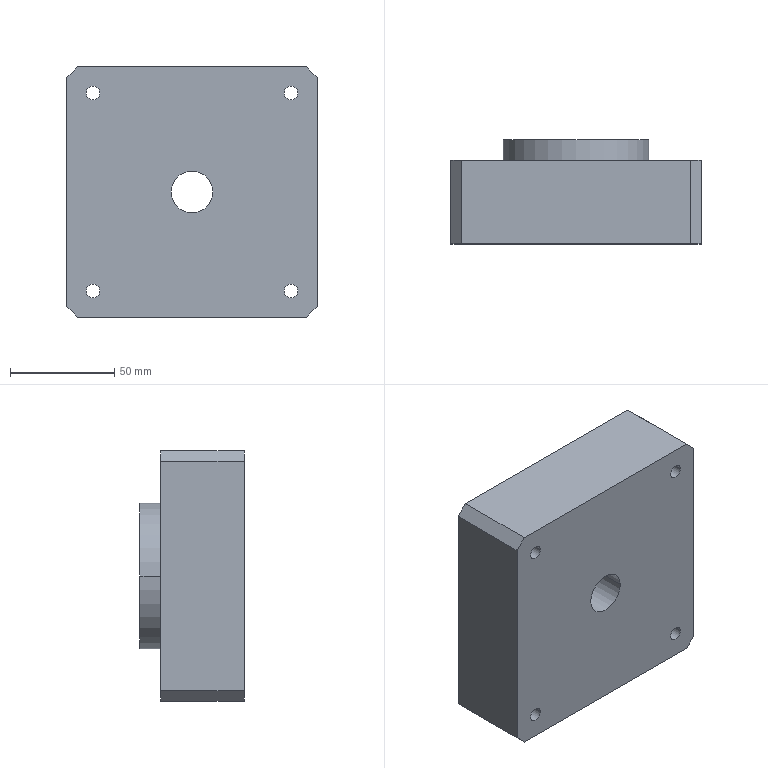Part | STEP file | M6 六角头Screw的柱形沉头Hole 1 | 1 solid | 50 faces | box 120 x 50 x 120 mm | volume 583267 mm3 | cylinder 30 | plane 20 | commonest cylinder face diameters 6 x8 6.6 x8 14.55 x8 20 x2 40 x2 70 x2
STEP:
#1=CARTESIAN_POINT('',(-1528.963,1730.114,2864.251));
#2=VERTEX_POINT('',#1);
#3=CARTESIAN_POINT('',(-1543.513,1730.114,2864.251));
#4=VERTEX_POINT('',#3);
#5=CARTESIAN_POINT('',(-1536.238,1730.114,2864.251));
#6=DIRECTION('',(0.,1.,0.));
#7=DIRECTION('',(-1.,0.,0.));
#8=AXIS2_PLACEMENT_3D('',#5,#6,#7);
#9=CIRCLE('',#8,7.275);
#10=EDGE_CURVE('',#2,#4,#9,.T.);
#11=ORIENTED_EDGE('',*,*,#10,.F.);
#12=CARTESIAN_POINT('',(-1528.963,1734.264,2864.251));
#13=VERTEX_POINT('',#12);
#14=CARTESIAN_POINT('',(-1528.963,1734.264,2864.251));
#15=DIRECTION('',(0.,1.,0.));
#16=VECTOR('',#15,1000.);
#17=LINE('',#14,#16);
#18=EDGE_CURVE('',#2,#13,#17,.T.);
#19=ORIENTED_EDGE('',*,*,#18,.T.);
#20=CARTESIAN_POINT('',(-1543.513,1734.264,2864.251));
#21=VERTEX_POINT('',#20);
#22=CARTESIAN_POINT('',(-1536.238,1734.264,2864.251));
#23=DIRECTION('',(0.,1.,0.));
#24=DIRECTION('',(-1.,0.,0.));
#25=AXIS2_PLACEMENT_3D('',#22,#23,#24);
#26=CIRCLE('',#25,7.275);
#27=EDGE_CURVE('',#13,#21,#26,.T.);
#28=ORIENTED_EDGE('',*,*,#27,.T.);
#29=CARTESIAN_POINT('',(-1543.513,1734.264,2864.251));
#30=DIRECTION('',(0.,1.,0.));
#31=VECTOR('',#30,1000.);
#32=LINE('',#29,#31);
#33=EDGE_CURVE('',#4,#21,#32,.T.);
#34=ORIENTED_EDGE('',*,*,#33,.F.);
#35=EDGE_LOOP('',(#11,#19,#28,#34));
#36=FACE_OUTER_BOUND('',#35,.T.);
#37=CARTESIAN_POINT('',(-1536.238,1734.264,2864.251));
#38=DIRECTION('',(0.,1.,0.));
#39=DIRECTION('',(1.,0.,0.));
#40=AXIS2_PLACEMENT_3D('',#37,#38,#39);
#41=CYLINDRICAL_SURFACE('',#40,7.275);
#42=ADVANCED_FACE('',(#36),#41,.F.);
#43=CARTESIAN_POINT('',(-1532.938,1694.264,2864.251));
#44=VERTEX_POINT('',#43);
#45=CARTESIAN_POINT('',(-1539.538,1694.264,2864.251));
#46=VERTEX_POINT('',#45);
#47=CARTESIAN_POINT('',(-1536.238,1694.264,2864.251));
#48=DIRECTION('',(0.,1.,0.));
#49=DIRECTION('',(-1.,0.,0.));
#50=AXIS2_PLACEMENT_3D('',#47,#48,#49);
#51=CIRCLE('',#50,3.3);
#52=EDGE_CURVE('',#44,#46,#51,.T.);
#53=ORIENTED_EDGE('',*,*,#52,.F.);
#54=CARTESIAN_POINT('',(-1532.938,1730.114,2864.251));
#55=VERTEX_POINT('',#54);
#56=CARTESIAN_POINT('',(-1532.938,1734.264,2864.251));
#57=DIRECTION('',(0.,1.,0.));
#58=VECTOR('',#57,1000.);
#59=LINE('',#56,#58);
#60=EDGE_CURVE('',#44,#55,#59,.T.);
#61=ORIENTED_EDGE('',*,*,#60,.T.);
#62=CARTESIAN_POINT('',(-1539.538,1730.114,2864.251));
#63=VERTEX_POINT('',#62);
#64=CARTESIAN_POINT('',(-1536.238,1730.114,2864.251));
#65=DIRECTION('',(0.,1.,0.));
#66=DIRECTION('',(-1.,0.,0.));
#67=AXIS2_PLACEMENT_3D('',#64,#65,#66);
#68=CIRCLE('',#67,3.3);
#69=EDGE_CURVE('',#55,#63,#68,.T.);
#70=ORIENTED_EDGE('',*,*,#69,.T.);
#71=CARTESIAN_POINT('',(-1539.538,1734.264,2864.251));
#72=DIRECTION('',(0.,1.,0.));
#73=VECTOR('',#72,1000.);
#74=LINE('',#71,#73);
#75=EDGE_CURVE('',#46,#63,#74,.T.);
#76=ORIENTED_EDGE('',*,*,#75,.F.);
#77=EDGE_LOOP('',(#53,#61,#70,#76));
#78=FACE_OUTER_BOUND('',#77,.T.);
#79=CARTESIAN_POINT('',(-1536.238,1734.264,2864.251));
#80=DIRECTION('',(0.,1.,0.));
#81=DIRECTION('',(1.,0.,0.));
#82=AXIS2_PLACEMENT_3D('',#79,#80,#81);
#83=CYLINDRICAL_SURFACE('',#82,3.3);
#84=ADVANCED_FACE('',(#78),#83,.F.);
#85=CARTESIAN_POINT('',(-1433.963,1730.114,2769.251));
#86=VERTEX_POINT('',#85);
#87=CARTESIAN_POINT('',(-1448.513,1730.114,2769.251));
#88=VERTEX_POINT('',#87);
#89=CARTESIAN_POINT('',(-1441.238,1730.114,2769.251));
#90=DIRECTION('',(0.,1.,0.));
#91=DIRECTION('',(-1.,0.,0.));
#92=AXIS2_PLACEMENT_3D('',#89,#90,#91);
#93=CIRCLE('',#92,7.275);
#94=EDGE_CURVE('',#86,#88,#93,.T.);
#95=ORIENTED_EDGE('',*,*,#94,.F.);
#96=CARTESIAN_POINT('',(-1433.963,1734.264,2769.251));
#97=VERTEX_POINT('',#96);
#98=CARTESIAN_POINT('',(-1433.963,1734.264,2769.251));
#99=DIRECTION('',(0.,1.,0.));
#100=VECTOR('',#99,1000.);
#101=LINE('',#98,#100);
#102=EDGE_CURVE('',#86,#97,#101,.T.);
#103=ORIENTED_EDGE('',*,*,#102,.T.);
#104=CARTESIAN_POINT('',(-1448.513,1734.264,2769.251));
#105=VERTEX_POINT('',#104);
#106=CARTESIAN_POINT('',(-1441.238,1734.264,2769.251));
#107=DIRECTION('',(0.,1.,0.));
#108=DIRECTION('',(-1.,0.,0.));
#109=AXIS2_PLACEMENT_3D('',#106,#107,#108);
#110=CIRCLE('',#109,7.275);
#111=EDGE_CURVE('',#97,#105,#110,.T.);
#112=ORIENTED_EDGE('',*,*,#111,.T.);
#113=CARTESIAN_POINT('',(-1448.513,1734.264,2769.251));
#114=DIRECTION('',(0.,1.,0.));
#115=VECTOR('',#114,1000.);
#116=LINE('',#113,#115);
#117=EDGE_CURVE('',#88,#105,#116,.T.);
#118=ORIENTED_EDGE('',*,*,#117,.F.);
#119=EDGE_LOOP('',(#95,#103,#112,#118));
#120=FACE_OUTER_BOUND('',#119,.T.);
#121=CARTESIAN_POINT('',(-1441.238,1734.264,2769.251));
#122=DIRECTION('',(0.,1.,0.));
#123=DIRECTION('',(1.,0.,0.));
#124=AXIS2_PLACEMENT_3D('',#121,#122,#123);
#125=CYLINDRICAL_SURFACE('',#124,7.275);
#126=ADVANCED_FACE('',(#120),#125,.F.);
#127=CARTESIAN_POINT('',(-1437.938,1694.264,2769.251));
#128=VERTEX_POINT('',#127);
#129=CARTESIAN_POINT('',(-1444.538,1694.264,2769.251));
#130=VERTEX_POINT('',#129);
#131=CARTESIAN_POINT('',(-1441.238,1694.264,2769.251));
#132=DIRECTION('',(0.,1.,0.));
#133=DIRECTION('',(-1.,0.,0.));
#134=AXIS2_PLACEMENT_3D('',#131,#132,#133);
#135=CIRCLE('',#134,3.3);
#136=EDGE_CURVE('',#128,#130,#135,.T.);
#137=ORIENTED_EDGE('',*,*,#136,.F.);
#138=CARTESIAN_POINT('',(-1437.938,1730.114,2769.251));
#139=VERTEX_POINT('',#138);
#140=CARTESIAN_POINT('',(-1437.938,1734.264,2769.251));
#141=DIRECTION('',(0.,1.,0.));
#142=VECTOR('',#141,1000.);
#143=LINE('',#140,#142);
#144=EDGE_CURVE('',#128,#139,#143,.T.);
#145=ORIENTED_EDGE('',*,*,#144,.T.);
#146=CARTESIAN_POINT('',(-1444.538,1730.114,2769.251));
#147=VERTEX_POINT('',#146);
#148=CARTESIAN_POINT('',(-1441.238,1730.114,2769.251));
#149=DIRECTION('',(0.,1.,0.));
#150=DIRECTION('',(-1.,0.,0.));
#151=AXIS2_PLACEMENT_3D('',#148,#149,#150);
#152=CIRCLE('',#151,3.3);
#153=EDGE_CURVE('',#139,#147,#152,.T.);
#154=ORIENTED_EDGE('',*,*,#153,.T.);
#155=CARTESIAN_POINT('',(-1444.538,1734.264,2769.251));
#156=DIRECTION('',(0.,1.,0.));
#157=VECTOR('',#156,1000.);
#158=LINE('',#155,#157);
#159=EDGE_CURVE('',#130,#147,#158,.T.);
#160=ORIENTED_EDGE('',*,*,#159,.F.);
#161=EDGE_LOOP('',(#137,#145,#154,#160));
#162=FACE_OUTER_BOUND('',#161,.T.);
#163=CARTESIAN_POINT('',(-1441.238,1734.264,2769.251));
#164=DIRECTION('',(0.,1.,0.));
#165=DIRECTION('',(1.,0.,0.));
#166=AXIS2_PLACEMENT_3D('',#163,#164,#165);
#167=CYLINDRICAL_SURFACE('',#166,3.3);
#168=ADVANCED_FACE('',(#162),#167,.F.);
#169=CARTESIAN_POINT('',(-1433.963,1730.114,2864.251));
#170=VERTEX_POINT('',#169);
#171=CARTESIAN_POINT('',(-1448.513,1730.114,2864.251));
#172=VERTEX_POINT('',#171);
#173=CARTESIAN_POINT('',(-1441.238,1730.114,2864.251));
#174=DIRECTION('',(0.,1.,0.));
#175=DIRECTION('',(-1.,0.,0.));
#176=AXIS2_PLACEMENT_3D('',#173,#174,#175);
#177=CIRCLE('',#176,7.275);
#178=EDGE_CURVE('',#170,#172,#177,.T.);
#179=ORIENTED_EDGE('',*,*,#178,.F.);
#180=CARTESIAN_POINT('',(-1433.963,1734.264,2864.251));
#181=VERTEX_POINT('',#180);
#182=CARTESIAN_POINT('',(-1433.963,1734.264,2864.251));
#183=DIRECTION('',(0.,1.,0.));
#184=VECTOR('',#183,1000.);
#185=LINE('',#182,#184);
#186=EDGE_CURVE('',#170,#181,#185,.T.);
#187=ORIENTED_EDGE('',*,*,#186,.T.);
#188=CARTESIAN_POINT('',(-1448.513,1734.264,2864.251));
#189=VERTEX_POINT('',#188);
#190=CARTESIAN_POINT('',(-1441.238,1734.264,2864.251));
#191=DIRECTION('',(0.,1.,0.));
#192=DIRECTION('',(-1.,0.,0.));
#193=AXIS2_PLACEMENT_3D('',#190,#191,#192);
#194=CIRCLE('',#193,7.275);
#195=EDGE_CURVE('',#181,#189,#194,.T.);
#196=ORIENTED_EDGE('',*,*,#195,.T.);
#197=CARTESIAN_POINT('',(-1448.513,1734.264,2864.251));
#198=DIRECTION('',(0.,1.,0.));
#199=VECTOR('',#198,1000.);
#200=LINE('',#197,#199);
#201=EDGE_CURVE('',#172,#189,#200,.T.);
#202=ORIENTED_EDGE('',*,*,#201,.F.);
#203=EDGE_LOOP('',(#179,#187,#196,#202));
#204=FACE_OUTER_BOUND('',#203,.T.);
#205=CARTESIAN_POINT('',(-1441.238,1734.264,2864.251));
#206=DIRECTION('',(0.,1.,0.));
#207=DIRECTION('',(1.,0.,0.));
#208=AXIS2_PLACEMENT_3D('',#205,#206,#207);
#209=CYLINDRICAL_SURFACE('',#208,7.275);
#210=ADVANCED_FACE('',(#204),#209,.F.);
#211=CARTESIAN_POINT('',(-1437.938,1694.264,2864.251));
#212=VERTEX_POINT('',#211);
#213=CARTESIAN_POINT('',(-1444.538,1694.264,2864.251));
#214=VERTEX_POINT('',#213);
#215=CARTESIAN_POINT('',(-1441.238,1694.264,2864.251));
#216=DIRECTION('',(0.,1.,0.));
#217=DIRECTION('',(-1.,0.,0.));
#218=AXIS2_PLACEMENT_3D('',#215,#216,#217);
#219=CIRCLE('',#218,3.3);
#220=EDGE_CURVE('',#212,#214,#219,.T.);
#221=ORIENTED_EDGE('',*,*,#220,.F.);
#222=CARTESIAN_POINT('',(-1437.938,1730.114,2864.251));
#223=VERTEX_POINT('',#222);
#224=CARTESIAN_POINT('',(-1437.938,1734.264,2864.251));
#225=DIRECTION('',(0.,1.,0.));
#226=VECTOR('',#225,1000.);
#227=LINE('',#224,#226);
#228=EDGE_CURVE('',#212,#223,#227,.T.);
#229=ORIENTED_EDGE('',*,*,#228,.T.);
#230=CARTESIAN_POINT('',(-1444.538,1730.114,2864.251));
#231=VERTEX_POINT('',#230);
#232=CARTESIAN_POINT('',(-1441.238,1730.114,2864.251));
#233=DIRECTION('',(0.,1.,0.));
#234=DIRECTION('',(-1.,0.,0.));
#235=AXIS2_PLACEMENT_3D('',#232,#233,#234);
#236=CIRCLE('',#235,3.3);
#237=EDGE_CURVE('',#223,#231,#236,.T.);
#238=ORIENTED_EDGE('',*,*,#237,.T.);
#239=CARTESIAN_POINT('',(-1444.538,1734.264,2864.251));
#240=DIRECTION('',(0.,1.,0.));
#241=VECTOR('',#240,1000.);
#242=LINE('',#239,#241);
#243=EDGE_CURVE('',#214,#231,#242,.T.);
#244=ORIENTED_EDGE('',*,*,#243,.F.);
#245=EDGE_LOOP('',(#221,#229,#238,#244));
#246=FACE_OUTER_BOUND('',#245,.T.);
#247=CARTESIAN_POINT('',(-1441.238,1734.264,2864.251));
#248=DIRECTION('',(0.,1.,0.));
#249=DIRECTION('',(1.,0.,0.));
#250=AXIS2_PLACEMENT_3D('',#247,#248,#249);
#251=CYLINDRICAL_SURFACE('',#250,3.3);
#252=ADVANCED_FACE('',(#246),#251,.F.);
#253=CARTESIAN_POINT('',(-1528.963,1730.114,2769.251));
#254=VERTEX_POINT('',#253);
#255=CARTESIAN_POINT('',(-1543.513,1730.114,2769.251));
#256=VERTEX_POINT('',#255);
#257=CARTESIAN_POINT('',(-1536.238,1730.114,2769.251));
#258=DIRECTION('',(0.,1.,0.));
#259=DIRECTION('',(-1.,0.,0.));
#260=AXIS2_PLACEMENT_3D('',#257,#258,#259);
#261=CIRCLE('',#260,7.275);
#262=EDGE_CURVE('',#254,#256,#261,.T.);
#263=ORIENTED_EDGE('',*,*,#262,.F.);
#264=CARTESIAN_POINT('',(-1528.963,1734.264,2769.251));
#265=VERTEX_POINT('',#264);
#266=CARTESIAN_POINT('',(-1528.963,1734.264,2769.251));
#267=DIRECTION('',(0.,1.,0.));
#268=VECTOR('',#267,1000.);
#269=LINE('',#266,#268);
#270=EDGE_CURVE('',#254,#265,#269,.T.);
#271=ORIENTED_EDGE('',*,*,#270,.T.);
#272=CARTESIAN_POINT('',(-1543.513,1734.264,2769.251));
#273=VERTEX_POINT('',#272);
#274=CARTESIAN_POINT('',(-1536.238,1734.264,2769.251));
#275=DIRECTION('',(0.,1.,0.));
#276=DIRECTION('',(-1.,0.,0.));
#277=AXIS2_PLACEMENT_3D('',#274,#275,#276);
#278=CIRCLE('',#277,7.275);
#279=EDGE_CURVE('',#265,#273,#278,.T.);
#280=ORIENTED_EDGE('',*,*,#279,.T.);
#281=CARTESIAN_POINT('',(-1543.513,1734.264,2769.251));
#282=DIRECTION('',(0.,1.,0.));
#283=VECTOR('',#282,1000.);
#284=LINE('',#281,#283);
#285=EDGE_CURVE('',#256,#273,#284,.T.);
#286=ORIENTED_EDGE('',*,*,#285,.F.);
#287=EDGE_LOOP('',(#263,#271,#280,#286));
#288=FACE_OUTER_BOUND('',#287,.T.);
#289=CARTESIAN_POINT('',(-1536.238,1734.264,2769.251));
#290=DIRECTION('',(0.,1.,0.));
#291=DIRECTION('',(1.,0.,0.));
#292=AXIS2_PLACEMENT_3D('',#289,#290,#291);
#293=CYLINDRICAL_SURFACE('',#292,7.275);
#294=ADVANCED_FACE('',(#288),#293,.F.);
#295=CARTESIAN_POINT('',(-1532.938,1694.264,2769.251));
#296=VERTEX_POINT('',#295);
#297=CARTESIAN_POINT('',(-1539.538,1694.264,2769.251));
#298=VERTEX_POINT('',#297);
#299=CARTESIAN_POINT('',(-1536.238,1694.264,2769.251));
#300=DIRECTION('',(0.,1.,0.));
#301=DIRECTION('',(-1.,0.,0.));
#302=AXIS2_PLACEMENT_3D('',#299,#300,#301);
#303=CIRCLE('',#302,3.3);
#304=EDGE_CURVE('',#296,#298,#303,.T.);
#305=ORIENTED_EDGE('',*,*,#304,.F.);
#306=CARTESIAN_POINT('',(-1532.938,1730.114,2769.251));
#307=VERTEX_POINT('',#306);
#308=CARTESIAN_POINT('',(-1532.938,1734.264,2769.251));
#309=DIRECTION('',(0.,1.,0.));
#310=VECTOR('',#309,1000.);
#311=LINE('',#308,#310);
#312=EDGE_CURVE('',#296,#307,#311,.T.);
#313=ORIENTED_EDGE('',*,*,#312,.T.);
#314=CARTESIAN_POINT('',(-1539.538,1730.114,2769.251));
#315=VERTEX_POINT('',#314);
#316=CARTESIAN_POINT('',(-1536.238,1730.114,2769.251));
#317=DIRECTION('',(0.,1.,0.));
#318=DIRECTION('',(-1.,0.,0.));
#319=AXIS2_PLACEMENT_3D('',#316,#317,#318);
#320=CIRCLE('',#319,3.3);
#321=EDGE_CURVE('',#307,#315,#320,.T.);
#322=ORIENTED_EDGE('',*,*,#321,.T.);
#323=CARTESIAN_POINT('',(-1539.538,1734.264,2769.251));
#324=DIRECTION('',(0.,1.,0.));
#325=VECTOR('',#324,1000.);
#326=LINE('',#323,#325);
#327=EDGE_CURVE('',#298,#315,#326,.T.);
#328=ORIENTED_EDGE('',*,*,#327,.F.);
#329=EDGE_LOOP('',(#305,#313,#322,#328));
#330=FACE_OUTER_BOUND('',#329,.T.);
#331=CARTESIAN_POINT('',(-1536.238,1734.264,2769.251));
#332=DIRECTION('',(0.,1.,0.));
#333=DIRECTION('',(1.,0.,0.));
#334=AXIS2_PLACEMENT_3D('',#331,#332,#333);
#335=CYLINDRICAL_SURFACE('',#334,3.3);
#336=ADVANCED_FACE('',(#330),#335,.F.);
#337=CARTESIAN_POINT('',(-1515.738,1724.264,2786.751));
#338=VERTEX_POINT('',#337);
#339=CARTESIAN_POINT('',(-1521.738,1724.264,2786.751));
#340=VERTEX_POINT('',#339);
#341=CARTESIAN_POINT('',(-1518.738,1724.264,2786.751));
#342=DIRECTION('',(0.,1.,0.));
#343=DIRECTION('',(-1.,0.,0.));
#344=AXIS2_PLACEMENT_3D('',#341,#342,#343);
#345=CIRCLE('',#344,3.);
#346=EDGE_CURVE('',#338,#340,#345,.T.);
#347=ORIENTED_EDGE('',*,*,#346,.F.);
#348=CARTESIAN_POINT('',(-1515.738,1734.264,2786.751));
#349=VERTEX_POINT('',#348);
#350=CARTESIAN_POINT('',(-1515.738,1724.264,2786.751));
#351=DIRECTION('',(0.,1.,0.));
#352=VECTOR('',#351,1000.);
#353=LINE('',#350,#352);
#354=EDGE_CURVE('',#338,#349,#353,.T.);
#355=ORIENTED_EDGE('',*,*,#354,.T.);
#356=CARTESIAN_POINT('',(-1521.738,1734.264,2786.751));
#357=VERTEX_POINT('',#356);
#358=CARTESIAN_POINT('',(-1518.738,1734.264,2786.751));
#359=DIRECTION('',(0.,1.,0.));
#360=DIRECTION('',(-1.,0.,0.));
#361=AXIS2_PLACEMENT_3D('',#358,#359,#360);
#362=CIRCLE('',#361,3.);
#363=EDGE_CURVE('',#349,#357,#362,.T.);
#364=ORIENTED_EDGE('',*,*,#363,.T.);
#365=CARTESIAN_POINT('',(-1521.738,1724.264,2786.751));
#366=DIRECTION('',(0.,1.,0.));
#367=VECTOR('',#366,1000.);
#368=LINE('',#365,#367);
#369=EDGE_CURVE('',#340,#357,#368,.T.);
#370=ORIENTED_EDGE('',*,*,#369,.F.);
#371=EDGE_LOOP('',(#347,#355,#364,#370));
#372=FACE_OUTER_BOUND('',#371,.T.);
#373=CARTESIAN_POINT('',(-1518.738,1724.264,2786.751));
#374=DIRECTION('',(0.,1.,0.));
#375=DIRECTION('',(1.,0.,0.));
#376=AXIS2_PLACEMENT_3D('',#373,#374,#375);
#377=CYLINDRICAL_SURFACE('',#376,3.);
#378=ADVANCED_FACE('',(#372),#377,.F.);
#379=CARTESIAN_POINT('',(-1515.738,1724.264,2846.751));
#380=VERTEX_POINT('',#379);
#381=CARTESIAN_POINT('',(-1521.738,1724.264,2846.751));
#382=VERTEX_POINT('',#381);
#383=CARTESIAN_POINT('',(-1518.738,1724.264,2846.751));
#384=DIRECTION('',(0.,1.,0.));
#385=DIRECTION('',(-1.,0.,0.));
#386=AXIS2_PLACEMENT_3D('',#383,#384,#385);
#387=CIRCLE('',#386,3.);
#388=EDGE_CURVE('',#380,#382,#387,.T.);
#389=ORIENTED_EDGE('',*,*,#388,.F.);
#390=CARTESIAN_POINT('',(-1515.738,1734.264,2846.751));
#391=VERTEX_POINT('',#390);
#392=CARTESIAN_POINT('',(-1515.738,1724.264,2846.751));
#393=DIRECTION('',(0.,1.,0.));
#394=VECTOR('',#393,1000.);
#395=LINE('',#392,#394);
#396=EDGE_CURVE('',#380,#391,#395,.T.);
#397=ORIENTED_EDGE('',*,*,#396,.T.);
#398=CARTESIAN_POINT('',(-1521.738,1734.264,2846.751));
#399=VERTEX_POINT('',#398);
#400=CARTESIAN_POINT('',(-1518.738,1734.264,2846.751));
#401=DIRECTION('',(0.,1.,0.));
#402=DIRECTION('',(-1.,0.,0.));
#403=AXIS2_PLACEMENT_3D('',#400,#401,#402);
#404=CIRCLE('',#403,3.);
#405=EDGE_CURVE('',#391,#399,#404,.T.);
#406=ORIENTED_EDGE('',*,*,#405,.T.);
#407=CARTESIAN_POINT('',(-1521.738,1724.264,2846.751));
#408=DIRECTION('',(0.,1.,0.));
#409=VECTOR('',#408,1000.);
#410=LINE('',#407,#409);
#411=EDGE_CURVE('',#382,#399,#410,.T.);
#412=ORIENTED_EDGE('',*,*,#411,.F.);
#413=EDGE_LOOP('',(#389,#397,#406,#412));
#414=FACE_OUTER_BOUND('',#413,.T.);
#415=CARTESIAN_POINT('',(-1518.738,1724.264,2846.751));
#416=DIRECTION('',(0.,1.,0.));
#417=DIRECTION('',(1.,0.,0.));
#418=AXIS2_PLACEMENT_3D('',#415,#416,#417);
#419=CYLINDRICAL_SURFACE('',#418,3.);
#420=ADVANCED_FACE('',(#414),#419,.F.);
#421=CARTESIAN_POINT('',(-1455.738,1724.264,2786.751));
#422=VERTEX_POINT('',#421);
#423=CARTESIAN_POINT('',(-1461.738,1724.264,2786.751));
#424=VERTEX_POINT('',#423);
#425=CARTESIAN_POINT('',(-1458.738,1724.264,2786.751));
#426=DIRECTION('',(0.,1.,0.));
#427=DIRECTION('',(-1.,0.,0.));
#428=AXIS2_PLACEMENT_3D('',#425,#426,#427);
#429=CIRCLE('',#428,3.);
#430=EDGE_CURVE('',#422,#424,#429,.T.);
#431=ORIENTED_EDGE('',*,*,#430,.F.);
#432=CARTESIAN_POINT('',(-1455.738,1734.264,2786.751));
#433=VERTEX_POINT('',#432);
#434=CARTESIAN_POINT('',(-1455.738,1724.264,2786.751));
#435=DIRECTION('',(0.,1.,0.));
#436=VECTOR('',#435,1000.);
#437=LINE('',#434,#436);
#438=EDGE_CURVE('',#422,#433,#437,.T.);
#439=ORIENTED_EDGE('',*,*,#438,.T.);
#440=CARTESIAN_POINT('',(-1461.738,1734.264,2786.751));
#441=VERTEX_POINT('',#440);
#442=CARTESIAN_POINT('',(-1458.738,1734.264,2786.751));
#443=DIRECTION('',(0.,1.,0.));
#444=DIRECTION('',(-1.,0.,0.));
#445=AXIS2_PLACEMENT_3D('',#442,#443,#444);
#446=CIRCLE('',#445,3.);
#447=EDGE_CURVE('',#433,#441,#446,.T.);
#448=ORIENTED_EDGE('',*,*,#447,.T.);
#449=CARTESIAN_POINT('',(-1461.738,1724.264,2786.751));
#450=DIRECTION('',(0.,1.,0.));
#451=VECTOR('',#450,1000.);
#452=LINE('',#449,#451);
#453=EDGE_CURVE('',#424,#441,#452,.T.);
#454=ORIENTED_EDGE('',*,*,#453,.F.);
#455=EDGE_LOOP('',(#431,#439,#448,#454));
#456=FACE_OUTER_BOUND('',#455,.T.);
#457=CARTESIAN_POINT('',(-1458.738,1724.264,2786.751));
#458=DIRECTION('',(0.,1.,0.));
#459=DIRECTION('',(1.,0.,0.));
#460=AXIS2_PLACEMENT_3D('',#457,#458,#459);
#461=CYLINDRICAL_SURFACE('',#460,3.);
#462=ADVANCED_FACE('',(#456),#461,.F.);
#463=CARTESIAN_POINT('',(-1455.738,1724.264,2846.751));
#464=VERTEX_POINT('',#463);
#465=CARTESIAN_POINT('',(-1461.738,1724.264,2846.751));
#466=VERTEX_POINT('',#465);
#467=CARTESIAN_POINT('',(-1458.738,1724.264,2846.751));
#468=DIRECTION('',(0.,1.,0.));
#469=DIRECTION('',(-1.,0.,0.));
#470=AXIS2_PLACEMENT_3D('',#467,#468,#469);
#471=CIRCLE('',#470,3.);
#472=EDGE_CURVE('',#464,#466,#471,.T.);
#473=ORIENTED_EDGE('',*,*,#472,.F.);
#474=CARTESIAN_POINT('',(-1455.738,1734.264,2846.751));
#475=VERTEX_POINT('',#474);
#476=CARTESIAN_POINT('',(-1455.738,1724.264,2846.751));
#477=DIRECTION('',(0.,1.,0.));
#478=VECTOR('',#477,1000.);
#479=LINE('',#476,#478);
#480=EDGE_CURVE('',#464,#475,#479,.T.);
#481=ORIENTED_EDGE('',*,*,#480,.T.);
#482=CARTESIAN_POINT('',(-1461.738,1734.264,2846.751));
#483=VERTEX_POINT('',#482);
#484=CARTESIAN_POINT('',(-1458.738,1734.264,2846.751));
#485=DIRECTION('',(0.,1.,0.));
#486=DIRECTION('',(-1.,0.,0.));
#487=AXIS2_PLACEMENT_3D('',#484,#485,#486);
#488=CIRCLE('',#487,3.);
#489=EDGE_CURVE('',#475,#483,#488,.T.);
#490=ORIENTED_EDGE('',*,*,#489,.T.);
#491=CARTESIAN_POINT('',(-1461.738,1724.264,2846.751));
#492=DIRECTION('',(0.,1.,0.));
#493=VECTOR('',#492,1000.);
#494=LINE('',#491,#493);
#495=EDGE_CURVE('',#466,#483,#494,.T.);
#496=ORIENTED_EDGE('',*,*,#495,.F.);
#497=EDGE_LOOP('',(#473,#481,#490,#496));
#498=FACE_OUTER_BOUND('',#497,.T.);
#499=CARTESIAN_POINT('',(-1458.738,1724.264,2846.751));
#500=DIRECTION('',(0.,1.,0.));
#501=DIRECTION('',(1.,0.,0.));
#502=AXIS2_PLACEMENT_3D('',#499,#500,#501);
#503=CYLINDRICAL_SURFACE('',#502,3.);
#504=ADVANCED_FACE('',(#498),#503,.F.);
#505=CARTESIAN_POINT('',(-1498.738,1694.264,2816.751));
#506=VERTEX_POINT('',#505);
#507=CARTESIAN_POINT('',(-1478.738,1694.264,2816.751));
#508=VERTEX_POINT('',#507);
#509=CARTESIAN_POINT('',(-1488.738,1694.264,2816.751));
#510=DIRECTION('',(0.,-1.,0.));
#511=DIRECTION('',(1.,0.,0.));
#512=AXIS2_PLACEMENT_3D('',#509,#510,#511);
#513=CIRCLE('',#512,10.);
#514=EDGE_CURVE('',#506,#508,#513,.T.);
#515=ORIENTED_EDGE('',*,*,#514,.T.);
#516=CARTESIAN_POINT('',(-1478.738,1739.264,2816.751));
#517=VERTEX_POINT('',#516);
#518=CARTESIAN_POINT('',(-1478.738,1650.264,2816.751));
#519=DIRECTION('',(0.,1.,0.));
#520=VECTOR('',#519,1000.);
#521=LINE('',#518,#520);
#522=EDGE_CURVE('',#508,#517,#521,.T.);
#523=ORIENTED_EDGE('',*,*,#522,.T.);
#524=CARTESIAN_POINT('',(-1498.738,1739.264,2816.751));
#525=VERTEX_POINT('',#524);
#526=CARTESIAN_POINT('',(-1488.738,1739.264,2816.751));
#527=DIRECTION('',(0.,1.,0.));
#528=DIRECTION('',(-1.,0.,0.));
#529=AXIS2_PLACEMENT_3D('',#526,#527,#528);
#530=CIRCLE('',#529,10.);
#531=EDGE_CURVE('',#517,#525,#530,.T.);
#532=ORIENTED_EDGE('',*,*,#531,.T.);
#533=CARTESIAN_POINT('',(-1498.738,1650.264,2816.751));
#534=DIRECTION('',(0.,1.,0.));
#535=VECTOR('',#534,1000.);
#536=LINE('',#533,#535);
#537=EDGE_CURVE('',#506,#525,#536,.T.);
#538=ORIENTED_EDGE('',*,*,#537,.F.);
#539=EDGE_LOOP('',(#515,#523,#532,#538));
#540=FACE_OUTER_BOUND('',#539,.T.);
#541=CARTESIAN_POINT('',(-1488.738,1650.264,2816.751));
#542=DIRECTION('',(0.,1.,0.));
#543=DIRECTION('',(1.,0.,0.));
#544=AXIS2_PLACEMENT_3D('',#541,#542,#543);
#545=CYLINDRICAL_SURFACE('',#544,10.);
#546=ADVANCED_FACE('',(#540),#545,.F.);
#547=CARTESIAN_POINT('',(-1468.738,1739.264,2816.751));
#548=VERTEX_POINT('',#547);
#549=CARTESIAN_POINT('',(-1508.738,1739.264,2816.751));
#550=VERTEX_POINT('',#549);
#551=CARTESIAN_POINT('',(-1488.738,1739.264,2816.751));
#552=DIRECTION('',(0.,1.,0.));
#553=DIRECTION('',(-1.,0.,0.));
#554=AXIS2_PLACEMENT_3D('',#551,#552,#553);
#555=CIRCLE('',#554,20.);
#556=EDGE_CURVE('',#548,#550,#555,.T.);
#557=ORIENTED_EDGE('',*,*,#556,.F.);
#558=CARTESIAN_POINT('',(-1468.738,1744.264,2816.751));
#559=VERTEX_POINT('',#558);
#560=CARTESIAN_POINT('',(-1468.738,1739.264,2816.751));
#561=DIRECTION('',(0.,1.,0.));
#562=VECTOR('',#561,1000.);
#563=LINE('',#560,#562);
#564=EDGE_CURVE('',#548,#559,#563,.T.);
#565=ORIENTED_EDGE('',*,*,#564,.T.);
#566=CARTESIAN_POINT('',(-1508.738,1744.264,2816.751));
#567=VERTEX_POINT('',#566);
#568=CARTESIAN_POINT('',(-1488.738,1744.264,2816.751));
#569=DIRECTION('',(0.,1.,0.));
#570=DIRECTION('',(-1.,0.,0.));
#571=AXIS2_PLACEMENT_3D('',#568,#569,#570);
#572=CIRCLE('',#571,20.);
#573=EDGE_CURVE('',#559,#567,#572,.T.);
#574=ORIENTED_EDGE('',*,*,#573,.T.);
#575=CARTESIAN_POINT('',(-1508.738,1739.264,2816.751));
#576=DIRECTION('',(0.,1.,0.));
#577=VECTOR('',#576,1000.);
#578=LINE('',#575,#577);
#579=EDGE_CURVE('',#550,#567,#578,.T.);
#580=ORIENTED_EDGE('',*,*,#579,.F.);
#581=EDGE_LOOP('',(#557,#565,#574,#580));
#582=FACE_OUTER_BOUND('',#581,.T.);
#583=CARTESIAN_POINT('',(-1488.738,1739.264,2816.751));
#584=DIRECTION('',(0.,1.,0.));
#585=DIRECTION('',(1.,0.,0.));
#586=AXIS2_PLACEMENT_3D('',#583,#584,#585);
#587=CYLINDRICAL_SURFACE('',#586,20.);
#588=ADVANCED_FACE('',(#582),#587,.F.);
#589=CARTESIAN_POINT('',(-1523.738,1744.264,2816.751));
#590=VERTEX_POINT('',#589);
#591=CARTESIAN_POINT('',(-1453.738,1744.264,2816.751));
#592=VERTEX_POINT('',#591);
#593=CARTESIAN_POINT('',(-1488.738,1744.264,2816.751));
#594=DIRECTION('',(0.,1.,0.));
#595=DIRECTION('',(-1.,0.,0.));
#596=AXIS2_PLACEMENT_3D('',#593,#594,#595);
#597=CIRCLE('',#596,35.);
#598=EDGE_CURVE('',#590,#592,#597,.T.);
#599=ORIENTED_EDGE('',*,*,#598,.F.);
#600=CARTESIAN_POINT('',(-1523.738,1734.264,2816.751));
#601=VERTEX_POINT('',#600);
#602=CARTESIAN_POINT('',(-1523.738,1744.264,2816.751));
#603=DIRECTION('',(0.,1.,0.));
#604=VECTOR('',#603,1000.);
#605=LINE('',#602,#604);
#606=EDGE_CURVE('',#601,#590,#605,.T.);
#607=ORIENTED_EDGE('',*,*,#606,.F.);
#608=CARTESIAN_POINT('',(-1453.738,1734.264,2816.751));
#609=VERTEX_POINT('',#608);
#610=CARTESIAN_POINT('',(-1488.738,1734.264,2816.751));
#611=DIRECTION('',(0.,1.,0.));
#612=DIRECTION('',(1.,0.,0.));
#613=AXIS2_PLACEMENT_3D('',#610,#611,#612);
#614=CIRCLE('',#613,35.);
#615=EDGE_CURVE('',#601,#609,#614,.T.);
#616=ORIENTED_EDGE('',*,*,#615,.T.);
#617=CARTESIAN_POINT('',(-1453.738,1744.264,2816.751));
#618=DIRECTION('',(0.,1.,0.));
#619=VECTOR('',#618,1000.);
#620=LINE('',#617,#619);
#621=EDGE_CURVE('',#609,#592,#620,.T.);
#622=ORIENTED_EDGE('',*,*,#621,.T.);
#623=EDGE_LOOP('',(#599,#607,#616,#622));
#624=FACE_OUTER_BOUND('',#623,.T.);
#625=CARTESIAN_POINT('',(-1488.738,1744.264,2816.751));
#626=DIRECTION('',(0.,-1.,0.));
#627=DIRECTION('',(-1.,0.,0.));
#628=AXIS2_PLACEMENT_3D('',#625,#626,#627);
#629=CYLINDRICAL_SURFACE('',#628,35.);
#630=ADVANCED_FACE('',(#624),#629,.T.);
#631=CARTESIAN_POINT('',(-1536.238,1734.264,2864.251));
#632=DIRECTION('',(0.,1.,0.));
#633=DIRECTION('',(-1.,0.,0.));
#634=AXIS2_PLACEMENT_3D('',#631,#632,#633);
#635=CIRCLE('',#634,7.275);
#636=EDGE_CURVE('',#21,#13,#635,.T.);
#637=ORIENTED_EDGE('',*,*,#636,.F.);
#638=ORIENTED_EDGE('',*,*,#27,.F.);
#639=EDGE_LOOP('',(#637,#638));
#640=FACE_BOUND('',#639,.T.);
#641=CARTESIAN_POINT('',(-1441.238,1734.264,2769.251));
#642=DIRECTION('',(0.,1.,0.));
#643=DIRECTION('',(-1.,0.,0.));
#644=AXIS2_PLACEMENT_3D('',#641,#642,#643);
#645=CIRCLE('',#644,7.275);
#646=EDGE_CURVE('',#105,#97,#645,.T.);
#647=ORIENTED_EDGE('',*,*,#646,.F.);
#648=ORIENTED_EDGE('',*,*,#111,.F.);
#649=EDGE_LOOP('',(#647,#648));
#650=FACE_BOUND('',#649,.T.);
#651=CARTESIAN_POINT('',(-1441.238,1734.264,2864.251));
#652=DIRECTION('',(0.,1.,0.));
#653=DIRECTION('',(-1.,0.,0.));
#654=AXIS2_PLACEMENT_3D('',#651,#652,#653);
#655=CIRCLE('',#654,7.275);
#656=EDGE_CURVE('',#189,#181,#655,.T.);
#657=ORIENTED_EDGE('',*,*,#656,.F.);
#658=ORIENTED_EDGE('',*,*,#195,.F.);
#659=EDGE_LOOP('',(#657,#658));
#660=FACE_BOUND('',#659,.T.);
#661=CARTESIAN_POINT('',(-1536.238,1734.264,2769.251));
#662=DIRECTION('',(0.,1.,0.));
#663=DIRECTION('',(-1.,0.,0.));
#664=AXIS2_PLACEMENT_3D('',#661,#662,#663);
#665=CIRCLE('',#664,7.275);
#666=EDGE_CURVE('',#273,#265,#665,.T.);
#667=ORIENTED_EDGE('',*,*,#666,.F.);
#668=ORIENTED_EDGE('',*,*,#279,.F.);
#669=EDGE_LOOP('',(#667,#668));
#670=FACE_BOUND('',#669,.T.);
#671=CARTESIAN_POINT('',(-1518.738,1734.264,2786.751));
#672=DIRECTION('',(0.,1.,0.));
#673=DIRECTION('',(-1.,0.,0.));
#674=AXIS2_PLACEMENT_3D('',#671,#672,#673);
#675=CIRCLE('',#674,3.);
#676=EDGE_CURVE('',#357,#349,#675,.T.);
#677=ORIENTED_EDGE('',*,*,#676,.F.);
#678=ORIENTED_EDGE('',*,*,#363,.F.);
#679=EDGE_LOOP('',(#677,#678));
#680=FACE_BOUND('',#679,.T.);
#681=CARTESIAN_POINT('',(-1518.738,1734.264,2846.751));
#682=DIRECTION('',(0.,1.,0.));
#683=DIRECTION('',(-1.,0.,0.));
#684=AXIS2_PLACEMENT_3D('',#681,#682,#683);
#685=CIRCLE('',#684,3.);
#686=EDGE_CURVE('',#399,#391,#685,.T.);
#687=ORIENTED_EDGE('',*,*,#686,.F.);
#688=ORIENTED_EDGE('',*,*,#405,.F.);
#689=EDGE_LOOP('',(#687,#688));
#690=FACE_BOUND('',#689,.T.);
#691=CARTESIAN_POINT('',(-1458.738,1734.264,2786.751));
#692=DIRECTION('',(0.,1.,0.));
#693=DIRECTION('',(-1.,0.,0.));
#694=AXIS2_PLACEMENT_3D('',#691,#692,#693);
#695=CIRCLE('',#694,3.);
#696=EDGE_CURVE('',#441,#433,#695,.T.);
#697=ORIENTED_EDGE('',*,*,#696,.F.);
#698=ORIENTED_EDGE('',*,*,#447,.F.);
#699=EDGE_LOOP('',(#697,#698));
#700=FACE_BOUND('',#699,.T.);
#701=CARTESIAN_POINT('',(-1458.738,1734.264,2846.751));
#702=DIRECTION('',(0.,1.,0.));
#703=DIRECTION('',(-1.,0.,0.));
#704=AXIS2_PLACEMENT_3D('',#701,#702,#703);
#705=CIRCLE('',#704,3.);
#706=EDGE_CURVE('',#483,#475,#705,.T.);
#707=ORIENTED_EDGE('',*,*,#706,.F.);
#708=ORIENTED_EDGE('',*,*,#489,.F.);
#709=EDGE_LOOP('',(#707,#708));
#710=FACE_BOUND('',#709,.T.);
#711=CARTESIAN_POINT('',(-1548.738,1734.264,2871.751));
#712=VERTEX_POINT('',#711);
#713=CARTESIAN_POINT('',(-1548.738,1734.264,2761.751));
#714=VERTEX_POINT('',#713);
#715=CARTESIAN_POINT('',(-1548.738,1734.264,2876.751));
#716=DIRECTION('',(0.,0.,-1.));
#717=VECTOR('',#716,1000.);
#718=LINE('',#715,#717);
#719=EDGE_CURVE('',#712,#714,#718,.T.);
#720=ORIENTED_EDGE('',*,*,#719,.F.);
#721=CARTESIAN_POINT('',(-1543.738,1734.264,2876.751));
#722=VERTEX_POINT('',#721);
#723=CARTESIAN_POINT('',(-1548.738,1734.264,2871.751));
#724=DIRECTION('',(0.7071,0.,0.7071));
#725=VECTOR('',#724,1000.);
#726=LINE('',#723,#725);
#727=EDGE_CURVE('',#712,#722,#726,.T.);
#728=ORIENTED_EDGE('',*,*,#727,.T.);
#729=CARTESIAN_POINT('',(-1433.738,1734.264,2876.751));
#730=VERTEX_POINT('',#729);
#731=CARTESIAN_POINT('',(-1548.738,1734.264,2876.751));
#732=DIRECTION('',(-1.,0.,0.));
#733=VECTOR('',#732,1000.);
#734=LINE('',#731,#733);
#735=EDGE_CURVE('',#730,#722,#734,.T.);
#736=ORIENTED_EDGE('',*,*,#735,.F.);
#737=CARTESIAN_POINT('',(-1428.738,1734.264,2871.751));
#738=VERTEX_POINT('',#737);
#739=CARTESIAN_POINT('',(-1433.738,1734.264,2876.751));
#740=DIRECTION('',(0.7071,0.,-0.7071));
#741=VECTOR('',#740,1000.);
#742=LINE('',#739,#741);
#743=EDGE_CURVE('',#730,#738,#742,.T.);
#744=ORIENTED_EDGE('',*,*,#743,.T.);
#745=CARTESIAN_POINT('',(-1428.738,1734.264,2761.751));
#746=VERTEX_POINT('',#745);
#747=CARTESIAN_POINT('',(-1428.738,1734.264,2876.751));
#748=DIRECTION('',(0.,0.,1.));
#749=VECTOR('',#748,1000.);
#750=LINE('',#747,#749);
#751=EDGE_CURVE('',#746,#738,#750,.T.);
#752=ORIENTED_EDGE('',*,*,#751,.F.);
#753=CARTESIAN_POINT('',(-1433.738,1734.264,2756.751));
#754=VERTEX_POINT('',#753);
#755=CARTESIAN_POINT('',(-1428.738,1734.264,2761.751));
#756=DIRECTION('',(-0.7071,0.,-0.7071));
#757=VECTOR('',#756,1000.);
#758=LINE('',#755,#757);
#759=EDGE_CURVE('',#746,#754,#758,.T.);
#760=ORIENTED_EDGE('',*,*,#759,.T.);
#761=CARTESIAN_POINT('',(-1543.738,1734.264,2756.751));
#762=VERTEX_POINT('',#761);
#763=CARTESIAN_POINT('',(-1548.738,1734.264,2756.751));
#764=DIRECTION('',(1.,0.,0.));
#765=VECTOR('',#764,1000.);
#766=LINE('',#763,#765);
#767=EDGE_CURVE('',#762,#754,#766,.T.);
#768=ORIENTED_EDGE('',*,*,#767,.F.);
#769=CARTESIAN_POINT('',(-1543.738,1734.264,2756.751));
#770=DIRECTION('',(-0.7071,0.,0.7071));
#771=VECTOR('',#770,1000.);
#772=LINE('',#769,#771);
#773=EDGE_CURVE('',#762,#714,#772,.T.);
#774=ORIENTED_EDGE('',*,*,#773,.T.);
#775=EDGE_LOOP('',(#720,#728,#736,#744,#752,#760,#768,#774));
#776=FACE_OUTER_BOUND('',#775,.T.);
#777=CARTESIAN_POINT('',(-1488.738,1734.264,2816.751));
#778=DIRECTION('',(0.,1.,0.));
#779=DIRECTION('',(1.,0.,0.));
#780=AXIS2_PLACEMENT_3D('',#777,#778,#779);
#781=CIRCLE('',#780,35.);
#782=EDGE_CURVE('',#609,#601,#781,.T.);
#783=ORIENTED_EDGE('',*,*,#782,.F.);
#784=ORIENTED_EDGE('',*,*,#615,.F.);
#785=EDGE_LOOP('',(#783,#784));
#786=FACE_BOUND('',#785,.T.);
#787=CARTESIAN_POINT('',(-1488.738,1734.264,2816.751));
#788=DIRECTION('',(0.,-1.,0.));
#789=DIRECTION('',(-1.,0.,0.));
#790=AXIS2_PLACEMENT_3D('',#787,#788,#789);
#791=PLANE('',#790);
#792=ADVANCED_FACE('',(#640,#650,#660,#670,#680,#690,#700,#710,#776,#786),#791,.F.);
#793=CARTESIAN_POINT('',(-1428.738,1694.264,2761.751));
#794=VERTEX_POINT('',#793);
#795=CARTESIAN_POINT('',(-1428.738,1694.264,2871.751));
#796=VERTEX_POINT('',#795);
#797=CARTESIAN_POINT('',(-1428.738,1694.264,2876.751));
#798=DIRECTION('',(0.,0.,1.));
#799=VECTOR('',#798,1000.);
#800=LINE('',#797,#799);
#801=EDGE_CURVE('',#794,#796,#800,.T.);
#802=ORIENTED_EDGE('',*,*,#801,.F.);
#803=CARTESIAN_POINT('',(-1428.738,1694.264,2761.751));
#804=DIRECTION('',(0.,1.,0.));
#805=VECTOR('',#804,1000.);
#806=LINE('',#803,#805);
#807=EDGE_CURVE('',#794,#746,#806,.T.);
#808=ORIENTED_EDGE('',*,*,#807,.T.);
#809=ORIENTED_EDGE('',*,*,#751,.T.);
#810=CARTESIAN_POINT('',(-1428.738,1694.264,2871.751));
#811=DIRECTION('',(0.,-1.,0.));
#812=VECTOR('',#811,1000.);
#813=LINE('',#810,#812);
#814=EDGE_CURVE('',#738,#796,#813,.T.);
#815=ORIENTED_EDGE('',*,*,#814,.T.);
#816=EDGE_LOOP('',(#802,#808,#809,#815));
#817=FACE_OUTER_BOUND('',#816,.T.);
#818=CARTESIAN_POINT('',(-1428.738,1694.264,2876.751));
#819=DIRECTION('',(-1.,0.,0.));
#820=DIRECTION('',(0.,0.,1.));
#821=AXIS2_PLACEMENT_3D('',#818,#819,#820);
#822=PLANE('',#821);
#823=ADVANCED_FACE('',(#817),#822,.F.);
#824=ORIENTED_EDGE('',*,*,#735,.T.);
#825=CARTESIAN_POINT('',(-1543.738,1694.264,2876.751));
#826=VERTEX_POINT('',#825);
#827=CARTESIAN_POINT('',(-1543.738,1694.264,2876.751));
#828=DIRECTION('',(0.,-1.,0.));
#829=VECTOR('',#828,1000.);
#830=LINE('',#827,#829);
#831=EDGE_CURVE('',#722,#826,#830,.T.);
#832=ORIENTED_EDGE('',*,*,#831,.T.);
#833=CARTESIAN_POINT('',(-1433.738,1694.264,2876.751));
#834=VERTEX_POINT('',#833);
#835=CARTESIAN_POINT('',(-1548.738,1694.264,2876.751));
#836=DIRECTION('',(-1.,0.,0.));
#837=VECTOR('',#836,1000.);
#838=LINE('',#835,#837);
#839=EDGE_CURVE('',#834,#826,#838,.T.);
#840=ORIENTED_EDGE('',*,*,#839,.F.);
#841=CARTESIAN_POINT('',(-1433.738,1694.264,2876.751));
#842=DIRECTION('',(0.,1.,0.));
#843=VECTOR('',#842,1000.);
#844=LINE('',#841,#843);
#845=EDGE_CURVE('',#834,#730,#844,.T.);
#846=ORIENTED_EDGE('',*,*,#845,.T.);
#847=EDGE_LOOP('',(#824,#832,#840,#846));
#848=FACE_OUTER_BOUND('',#847,.T.);
#849=CARTESIAN_POINT('',(-1548.738,1694.264,2876.751));
#850=DIRECTION('',(0.,0.,-1.));
#851=DIRECTION('',(-1.,0.,0.));
#852=AXIS2_PLACEMENT_3D('',#849,#850,#851);
#853=PLANE('',#852);
#854=ADVANCED_FACE('',(#848),#853,.F.);
#855=CARTESIAN_POINT('',(-1548.738,1694.264,2871.751));
#856=VERTEX_POINT('',#855);
#857=CARTESIAN_POINT('',(-1548.738,1694.264,2761.751));
#858=VERTEX_POINT('',#857);
#859=CARTESIAN_POINT('',(-1548.738,1694.264,2876.751));
#860=DIRECTION('',(0.,0.,-1.));
#861=VECTOR('',#860,1000.);
#862=LINE('',#859,#861);
#863=EDGE_CURVE('',#856,#858,#862,.T.);
#864=ORIENTED_EDGE('',*,*,#863,.F.);
#865=CARTESIAN_POINT('',(-1548.738,1694.264,2871.751));
#866=DIRECTION('',(0.,1.,0.));
#867=VECTOR('',#866,1000.);
#868=LINE('',#865,#867);
#869=EDGE_CURVE('',#856,#712,#868,.T.);
#870=ORIENTED_EDGE('',*,*,#869,.T.);
#871=ORIENTED_EDGE('',*,*,#719,.T.);
#872=CARTESIAN_POINT('',(-1548.738,1694.264,2761.751));
#873=DIRECTION('',(0.,-1.,0.));
#874=VECTOR('',#873,1000.);
#875=LINE('',#872,#874);
#876=EDGE_CURVE('',#714,#858,#875,.T.);
#877=ORIENTED_EDGE('',*,*,#876,.T.);
#878=EDGE_LOOP('',(#864,#870,#871,#877));
#879=FACE_OUTER_BOUND('',#878,.T.);
#880=CARTESIAN_POINT('',(-1548.738,1694.264,2876.751));
#881=DIRECTION('',(1.,0.,0.));
#882=DIRECTION('',(0.,0.,-1.));
#883=AXIS2_PLACEMENT_3D('',#880,#881,#882);
#884=PLANE('',#883);
#885=ADVANCED_FACE('',(#879),#884,.F.);
#886=CARTESIAN_POINT('',(-1543.738,1694.264,2756.751));
#887=VERTEX_POINT('',#886);
#888=CARTESIAN_POINT('',(-1433.738,1694.264,2756.751));
#889=VERTEX_POINT('',#888);
#890=CARTESIAN_POINT('',(-1548.738,1694.264,2756.751));
#891=DIRECTION('',(1.,0.,0.));
#892=VECTOR('',#891,1000.);
#893=LINE('',#890,#892);
#894=EDGE_CURVE('',#887,#889,#893,.T.);
#895=ORIENTED_EDGE('',*,*,#894,.F.);
#896=CARTESIAN_POINT('',(-1543.738,1694.264,2756.751));
#897=DIRECTION('',(0.,1.,0.));
#898=VECTOR('',#897,1000.);
#899=LINE('',#896,#898);
#900=EDGE_CURVE('',#887,#762,#899,.T.);
#901=ORIENTED_EDGE('',*,*,#900,.T.);
#902=ORIENTED_EDGE('',*,*,#767,.T.);
#903=CARTESIAN_POINT('',(-1433.738,1694.264,2756.751));
#904=DIRECTION('',(0.,-1.,0.));
#905=VECTOR('',#904,1000.);
#906=LINE('',#903,#905);
#907=EDGE_CURVE('',#754,#889,#906,.T.);
#908=ORIENTED_EDGE('',*,*,#907,.T.);
#909=EDGE_LOOP('',(#895,#901,#902,#908));
#910=FACE_OUTER_BOUND('',#909,.T.);
#911=CARTESIAN_POINT('',(-1548.738,1694.264,2756.751));
#912=DIRECTION('',(0.,0.,1.));
#913=DIRECTION('',(1.,0.,0.));
#914=AXIS2_PLACEMENT_3D('',#911,#912,#913);
#915=PLANE('',#914);
#916=ADVANCED_FACE('',(#910),#915,.F.);
#917=CARTESIAN_POINT('',(-1536.238,1694.264,2864.251));
#918=DIRECTION('',(0.,1.,0.));
#919=DIRECTION('',(-1.,0.,0.));
#920=AXIS2_PLACEMENT_3D('',#917,#918,#919);
#921=CIRCLE('',#920,3.3);
#922=EDGE_CURVE('',#46,#44,#921,.T.);
#923=ORIENTED_EDGE('',*,*,#922,.T.);
#924=ORIENTED_EDGE('',*,*,#52,.T.);
#925=EDGE_LOOP('',(#923,#924));
#926=FACE_BOUND('',#925,.T.);
#927=CARTESIAN_POINT('',(-1441.238,1694.264,2769.251));
#928=DIRECTION('',(0.,1.,0.));
#929=DIRECTION('',(-1.,0.,0.));
#930=AXIS2_PLACEMENT_3D('',#927,#928,#929);
#931=CIRCLE('',#930,3.3);
#932=EDGE_CURVE('',#130,#128,#931,.T.);
#933=ORIENTED_EDGE('',*,*,#932,.T.);
#934=ORIENTED_EDGE('',*,*,#136,.T.);
#935=EDGE_LOOP('',(#933,#934));
#936=FACE_BOUND('',#935,.T.);
#937=CARTESIAN_POINT('',(-1441.238,1694.264,2864.251));
#938=DIRECTION('',(0.,1.,0.));
#939=DIRECTION('',(-1.,0.,0.));
#940=AXIS2_PLACEMENT_3D('',#937,#938,#939);
#941=CIRCLE('',#940,3.3);
#942=EDGE_CURVE('',#214,#212,#941,.T.);
#943=ORIENTED_EDGE('',*,*,#942,.T.);
#944=ORIENTED_EDGE('',*,*,#220,.T.);
#945=EDGE_LOOP('',(#943,#944));
#946=FACE_BOUND('',#945,.T.);
#947=CARTESIAN_POINT('',(-1536.238,1694.264,2769.251));
#948=DIRECTION('',(0.,1.,0.));
#949=DIRECTION('',(-1.,0.,0.));
#950=AXIS2_PLACEMENT_3D('',#947,#948,#949);
#951=CIRCLE('',#950,3.3);
#952=EDGE_CURVE('',#298,#296,#951,.T.);
#953=ORIENTED_EDGE('',*,*,#952,.T.);
#954=ORIENTED_EDGE('',*,*,#304,.T.);
#955=EDGE_LOOP('',(#953,#954));
#956=FACE_BOUND('',#955,.T.);
#957=ORIENTED_EDGE('',*,*,#514,.F.);
#958=CARTESIAN_POINT('',(-1488.738,1694.264,2816.751));
#959=DIRECTION('',(0.,-1.,0.));
#960=DIRECTION('',(1.,0.,0.));
#961=AXIS2_PLACEMENT_3D('',#958,#959,#960);
#962=CIRCLE('',#961,10.);
#963=EDGE_CURVE('',#508,#506,#962,.T.);
#964=ORIENTED_EDGE('',*,*,#963,.F.);
#965=EDGE_LOOP('',(#957,#964));
#966=FACE_BOUND('',#965,.T.);
#967=ORIENTED_EDGE('',*,*,#839,.T.);
#968=CARTESIAN_POINT('',(-1546.238,1694.264,2874.251));
#969=DIRECTION('',(-0.7071,0.,-0.7071));
#970=VECTOR('',#969,1000.);
#971=LINE('',#968,#970);
#972=EDGE_CURVE('',#826,#856,#971,.T.);
#973=ORIENTED_EDGE('',*,*,#972,.T.);
#974=ORIENTED_EDGE('',*,*,#863,.T.);
#975=CARTESIAN_POINT('',(-1546.238,1694.264,2759.251));
#976=DIRECTION('',(0.7071,0.,-0.7071));
#977=VECTOR('',#976,1000.);
#978=LINE('',#975,#977);
#979=EDGE_CURVE('',#858,#887,#978,.T.);
#980=ORIENTED_EDGE('',*,*,#979,.T.);
#981=ORIENTED_EDGE('',*,*,#894,.T.);
#982=CARTESIAN_POINT('',(-1431.238,1694.264,2759.251));
#983=DIRECTION('',(0.7071,0.,0.7071));
#984=VECTOR('',#983,1000.);
#985=LINE('',#982,#984);
#986=EDGE_CURVE('',#889,#794,#985,.T.);
#987=ORIENTED_EDGE('',*,*,#986,.T.);
#988=ORIENTED_EDGE('',*,*,#801,.T.);
#989=CARTESIAN_POINT('',(-1431.238,1694.264,2874.251));
#990=DIRECTION('',(-0.7071,0.,0.7071));
#991=VECTOR('',#990,1000.);
#992=LINE('',#989,#991);
#993=EDGE_CURVE('',#796,#834,#992,.T.);
#994=ORIENTED_EDGE('',*,*,#993,.T.);
#995=EDGE_LOOP('',(#967,#973,#974,#980,#981,#987,#988,#994));
#996=FACE_OUTER_BOUND('',#995,.T.);
#997=CARTESIAN_POINT('',(-1488.738,1694.264,2816.751));
#998=DIRECTION('',(0.,-1.,0.));
#999=DIRECTION('',(-1.,0.,0.));
#1000=AXIS2_PLACEMENT_3D('',#997,#998,#999);
#1001=PLANE('',#1000);
#1002=ADVANCED_FACE('',(#926,#936,#946,#956,#966,#996),#1001,.T.);
#1003=ORIENTED_EDGE('',*,*,#606,.T.);
#1004=CARTESIAN_POINT('',(-1488.738,1744.264,2816.751));
#1005=DIRECTION('',(0.,1.,0.));
#1006=DIRECTION('',(-1.,0.,0.));
#1007=AXIS2_PLACEMENT_3D('',#1004,#1005,#1006);
#1008=CIRCLE('',#1007,35.);
#1009=EDGE_CURVE('',#592,#590,#1008,.T.);
#1010=ORIENTED_EDGE('',*,*,#1009,.F.);
#1011=ORIENTED_EDGE('',*,*,#621,.F.);
#1012=ORIENTED_EDGE('',*,*,#782,.T.);
#1013=EDGE_LOOP('',(#1003,#1010,#1011,#1012));
#1014=FACE_OUTER_BOUND('',#1013,.T.);
#1015=CARTESIAN_POINT('',(-1488.738,1744.264,2816.751));
#1016=DIRECTION('',(0.,-1.,0.));
#1017=DIRECTION('',(-1.,0.,0.));
#1018=AXIS2_PLACEMENT_3D('',#1015,#1016,#1017);
#1019=CYLINDRICAL_SURFACE('',#1018,35.);
#1020=ADVANCED_FACE('',(#1014),#1019,.T.);
#1021=CARTESIAN_POINT('',(-1488.738,1744.264,2816.751));
#1022=DIRECTION('',(0.,1.,0.));
#1023=DIRECTION('',(-1.,0.,0.));
#1024=AXIS2_PLACEMENT_3D('',#1021,#1022,#1023);
#1025=CIRCLE('',#1024,20.);
#1026=EDGE_CURVE('',#567,#559,#1025,.T.);
#1027=ORIENTED_EDGE('',*,*,#1026,.F.);
#1028=ORIENTED_EDGE('',*,*,#573,.F.);
#1029=EDGE_LOOP('',(#1027,#1028));
#1030=FACE_BOUND('',#1029,.T.);
#1031=ORIENTED_EDGE('',*,*,#1009,.T.);
#1032=ORIENTED_EDGE('',*,*,#598,.T.);
#1033=EDGE_LOOP('',(#1031,#1032));
#1034=FACE_OUTER_BOUND('',#1033,.T.);
#1035=CARTESIAN_POINT('',(-1488.738,1744.264,2816.751));
#1036=DIRECTION('',(0.,1.,0.));
#1037=DIRECTION('',(1.,0.,0.));
#1038=AXIS2_PLACEMENT_3D('',#1035,#1036,#1037);
#1039=PLANE('',#1038);
#1040=ADVANCED_FACE('',(#1030,#1034),#1039,.T.);
#1041=ORIENTED_EDGE('',*,*,#564,.F.);
#1042=CARTESIAN_POINT('',(-1488.738,1739.264,2816.751));
#1043=DIRECTION('',(0.,1.,0.));
#1044=DIRECTION('',(-1.,0.,0.));
#1045=AXIS2_PLACEMENT_3D('',#1042,#1043,#1044);
#1046=CIRCLE('',#1045,20.);
#1047=EDGE_CURVE('',#550,#548,#1046,.T.);
#1048=ORIENTED_EDGE('',*,*,#1047,.F.);
#1049=ORIENTED_EDGE('',*,*,#579,.T.);
#1050=ORIENTED_EDGE('',*,*,#1026,.T.);
#1051=EDGE_LOOP('',(#1041,#1048,#1049,#1050));
#1052=FACE_OUTER_BOUND('',#1051,.T.);
#1053=CARTESIAN_POINT('',(-1488.738,1739.264,2816.751));
#1054=DIRECTION('',(0.,1.,0.));
#1055=DIRECTION('',(1.,0.,0.));
#1056=AXIS2_PLACEMENT_3D('',#1053,#1054,#1055);
#1057=CYLINDRICAL_SURFACE('',#1056,20.);
#1058=ADVANCED_FACE('',(#1052),#1057,.F.);
#1059=CARTESIAN_POINT('',(-1488.738,1739.264,2816.751));
#1060=DIRECTION('',(0.,1.,0.));
#1061=DIRECTION('',(-1.,0.,0.));
#1062=AXIS2_PLACEMENT_3D('',#1059,#1060,#1061);
#1063=CIRCLE('',#1062,10.);
#1064=EDGE_CURVE('',#525,#517,#1063,.T.);
#1065=ORIENTED_EDGE('',*,*,#1064,.F.);
#1066=ORIENTED_EDGE('',*,*,#531,.F.);
#1067=EDGE_LOOP('',(#1065,#1066));
#1068=FACE_BOUND('',#1067,.T.);
#1069=ORIENTED_EDGE('',*,*,#1047,.T.);
#1070=ORIENTED_EDGE('',*,*,#556,.T.);
#1071=EDGE_LOOP('',(#1069,#1070));
#1072=FACE_OUTER_BOUND('',#1071,.T.);
#1073=CARTESIAN_POINT('',(-1488.738,1739.264,2816.751));
#1074=DIRECTION('',(0.,1.,0.));
#1075=DIRECTION('',(1.,0.,0.));
#1076=AXIS2_PLACEMENT_3D('',#1073,#1074,#1075);
#1077=PLANE('',#1076);
#1078=ADVANCED_FACE('',(#1068,#1072),#1077,.T.);
#1079=ORIENTED_EDGE('',*,*,#972,.F.);
#1080=ORIENTED_EDGE('',*,*,#831,.F.);
#1081=ORIENTED_EDGE('',*,*,#727,.F.);
#1082=ORIENTED_EDGE('',*,*,#869,.F.);
#1083=EDGE_LOOP('',(#1079,#1080,#1081,#1082));
#1084=FACE_OUTER_BOUND('',#1083,.T.);
#1085=CARTESIAN_POINT('',(-1548.738,1694.264,2871.751));
#1086=DIRECTION('',(0.7071,0.,-0.7071));
#1087=DIRECTION('',(0.,-1.,0.));
#1088=AXIS2_PLACEMENT_3D('',#1085,#1086,#1087);
#1089=PLANE('',#1088);
#1090=ADVANCED_FACE('',(#1084),#1089,.F.);
#1091=ORIENTED_EDGE('',*,*,#979,.F.);
#1092=ORIENTED_EDGE('',*,*,#876,.F.);
#1093=ORIENTED_EDGE('',*,*,#773,.F.);
#1094=ORIENTED_EDGE('',*,*,#900,.F.);
#1095=EDGE_LOOP('',(#1091,#1092,#1093,#1094));
#1096=FACE_OUTER_BOUND('',#1095,.T.);
#1097=CARTESIAN_POINT('',(-1543.738,1694.264,2756.751));
#1098=DIRECTION('',(0.7071,0.,0.7071));
#1099=DIRECTION('',(0.,-1.,0.));
#1100=AXIS2_PLACEMENT_3D('',#1097,#1098,#1099);
#1101=PLANE('',#1100);
#1102=ADVANCED_FACE('',(#1096),#1101,.F.);
#1103=ORIENTED_EDGE('',*,*,#986,.F.);
#1104=ORIENTED_EDGE('',*,*,#907,.F.);
#1105=ORIENTED_EDGE('',*,*,#759,.F.);
#1106=ORIENTED_EDGE('',*,*,#807,.F.);
#1107=EDGE_LOOP('',(#1103,#1104,#1105,#1106));
#1108=FACE_OUTER_BOUND('',#1107,.T.);
#1109=CARTESIAN_POINT('',(-1428.738,1694.264,2761.751));
#1110=DIRECTION('',(-0.7071,0.,0.7071));
#1111=DIRECTION('',(0.,-1.,0.));
#1112=AXIS2_PLACEMENT_3D('',#1109,#1110,#1111);
#1113=PLANE('',#1112);
#1114=ADVANCED_FACE('',(#1108),#1113,.F.);
#1115=ORIENTED_EDGE('',*,*,#993,.F.);
#1116=ORIENTED_EDGE('',*,*,#814,.F.);
#1117=ORIENTED_EDGE('',*,*,#743,.F.);
#1118=ORIENTED_EDGE('',*,*,#845,.F.);
#1119=EDGE_LOOP('',(#1115,#1116,#1117,#1118));
#1120=FACE_OUTER_BOUND('',#1119,.T.);
#1121=CARTESIAN_POINT('',(-1433.738,1694.264,2876.751));
#1122=DIRECTION('',(-0.7071,0.,-0.7071));
#1123=DIRECTION('',(0.,-1.,0.));
#1124=AXIS2_PLACEMENT_3D('',#1121,#1122,#1123);
#1125=PLANE('',#1124);
#1126=ADVANCED_FACE('',(#1120),#1125,.F.);
#1127=ORIENTED_EDGE('',*,*,#522,.F.);
#1128=ORIENTED_EDGE('',*,*,#963,.T.);
#1129=ORIENTED_EDGE('',*,*,#537,.T.);
#1130=ORIENTED_EDGE('',*,*,#1064,.T.);
#1131=EDGE_LOOP('',(#1127,#1128,#1129,#1130));
#1132=FACE_OUTER_BOUND('',#1131,.T.);
#1133=CARTESIAN_POINT('',(-1488.738,1650.264,2816.751));
#1134=DIRECTION('',(0.,1.,0.));
#1135=DIRECTION('',(1.,0.,0.));
#1136=AXIS2_PLACEMENT_3D('',#1133,#1134,#1135);
#1137=CYLINDRICAL_SURFACE('',#1136,10.);
#1138=ADVANCED_FACE('',(#1132),#1137,.F.);
#1139=ORIENTED_EDGE('',*,*,#480,.F.);
#1140=CARTESIAN_POINT('',(-1458.738,1724.264,2846.751));
#1141=DIRECTION('',(0.,1.,0.));
#1142=DIRECTION('',(-1.,0.,0.));
#1143=AXIS2_PLACEMENT_3D('',#1140,#1141,#1142);
#1144=CIRCLE('',#1143,3.);
#1145=EDGE_CURVE('',#466,#464,#1144,.T.);
#1146=ORIENTED_EDGE('',*,*,#1145,.F.);
#1147=ORIENTED_EDGE('',*,*,#495,.T.);
#1148=ORIENTED_EDGE('',*,*,#706,.T.);
#1149=EDGE_LOOP('',(#1139,#1146,#1147,#1148));
#1150=FACE_OUTER_BOUND('',#1149,.T.);
#1151=CARTESIAN_POINT('',(-1458.738,1724.264,2846.751));
#1152=DIRECTION('',(0.,1.,0.));
#1153=DIRECTION('',(1.,0.,0.));
#1154=AXIS2_PLACEMENT_3D('',#1151,#1152,#1153);
#1155=CYLINDRICAL_SURFACE('',#1154,3.);
#1156=ADVANCED_FACE('',(#1150),#1155,.F.);
#1157=ORIENTED_EDGE('',*,*,#1145,.T.);
#1158=ORIENTED_EDGE('',*,*,#472,.T.);
#1159=EDGE_LOOP('',(#1157,#1158));
#1160=FACE_OUTER_BOUND('',#1159,.T.);
#1161=CARTESIAN_POINT('',(-1458.738,1724.264,2846.751));
#1162=DIRECTION('',(0.,1.,0.));
#1163=DIRECTION('',(1.,0.,0.));
#1164=AXIS2_PLACEMENT_3D('',#1161,#1162,#1163);
#1165=PLANE('',#1164);
#1166=ADVANCED_FACE('',(#1160),#1165,.T.);
#1167=ORIENTED_EDGE('',*,*,#438,.F.);
#1168=CARTESIAN_POINT('',(-1458.738,1724.264,2786.751));
#1169=DIRECTION('',(0.,1.,0.));
#1170=DIRECTION('',(-1.,0.,0.));
#1171=AXIS2_PLACEMENT_3D('',#1168,#1169,#1170);
#1172=CIRCLE('',#1171,3.);
#1173=EDGE_CURVE('',#424,#422,#1172,.T.);
#1174=ORIENTED_EDGE('',*,*,#1173,.F.);
#1175=ORIENTED_EDGE('',*,*,#453,.T.);
#1176=ORIENTED_EDGE('',*,*,#696,.T.);
#1177=EDGE_LOOP('',(#1167,#1174,#1175,#1176));
#1178=FACE_OUTER_BOUND('',#1177,.T.);
#1179=CARTESIAN_POINT('',(-1458.738,1724.264,2786.751));
#1180=DIRECTION('',(0.,1.,0.));
#1181=DIRECTION('',(1.,0.,0.));
#1182=AXIS2_PLACEMENT_3D('',#1179,#1180,#1181);
#1183=CYLINDRICAL_SURFACE('',#1182,3.);
#1184=ADVANCED_FACE('',(#1178),#1183,.F.);
#1185=ORIENTED_EDGE('',*,*,#1173,.T.);
#1186=ORIENTED_EDGE('',*,*,#430,.T.);
#1187=EDGE_LOOP('',(#1185,#1186));
#1188=FACE_OUTER_BOUND('',#1187,.T.);
#1189=CARTESIAN_POINT('',(-1458.738,1724.264,2786.751));
#1190=DIRECTION('',(0.,1.,0.));
#1191=DIRECTION('',(1.,0.,0.));
#1192=AXIS2_PLACEMENT_3D('',#1189,#1190,#1191);
#1193=PLANE('',#1192);
#1194=ADVANCED_FACE('',(#1188),#1193,.T.);
#1195=ORIENTED_EDGE('',*,*,#396,.F.);
#1196=CARTESIAN_POINT('',(-1518.738,1724.264,2846.751));
#1197=DIRECTION('',(0.,1.,0.));
#1198=DIRECTION('',(-1.,0.,0.));
#1199=AXIS2_PLACEMENT_3D('',#1196,#1197,#1198);
#1200=CIRCLE('',#1199,3.);
#1201=EDGE_CURVE('',#382,#380,#1200,.T.);
#1202=ORIENTED_EDGE('',*,*,#1201,.F.);
#1203=ORIENTED_EDGE('',*,*,#411,.T.);
#1204=ORIENTED_EDGE('',*,*,#686,.T.);
#1205=EDGE_LOOP('',(#1195,#1202,#1203,#1204));
#1206=FACE_OUTER_BOUND('',#1205,.T.);
#1207=CARTESIAN_POINT('',(-1518.738,1724.264,2846.751));
#1208=DIRECTION('',(0.,1.,0.));
#1209=DIRECTION('',(1.,0.,0.));
#1210=AXIS2_PLACEMENT_3D('',#1207,#1208,#1209);
#1211=CYLINDRICAL_SURFACE('',#1210,3.);
#1212=ADVANCED_FACE('',(#1206),#1211,.F.);
#1213=ORIENTED_EDGE('',*,*,#1201,.T.);
#1214=ORIENTED_EDGE('',*,*,#388,.T.);
#1215=EDGE_LOOP('',(#1213,#1214));
#1216=FACE_OUTER_BOUND('',#1215,.T.);
#1217=CARTESIAN_POINT('',(-1518.738,1724.264,2846.751));
#1218=DIRECTION('',(0.,1.,0.));
#1219=DIRECTION('',(1.,0.,0.));
#1220=AXIS2_PLACEMENT_3D('',#1217,#1218,#1219);
#1221=PLANE('',#1220);
#1222=ADVANCED_FACE('',(#1216),#1221,.T.);
#1223=ORIENTED_EDGE('',*,*,#354,.F.);
#1224=CARTESIAN_POINT('',(-1518.738,1724.264,2786.751));
#1225=DIRECTION('',(0.,1.,0.));
#1226=DIRECTION('',(-1.,0.,0.));
#1227=AXIS2_PLACEMENT_3D('',#1224,#1225,#1226);
#1228=CIRCLE('',#1227,3.);
#1229=EDGE_CURVE('',#340,#338,#1228,.T.);
#1230=ORIENTED_EDGE('',*,*,#1229,.F.);
#1231=ORIENTED_EDGE('',*,*,#369,.T.);
#1232=ORIENTED_EDGE('',*,*,#676,.T.);
#1233=EDGE_LOOP('',(#1223,#1230,#1231,#1232));
#1234=FACE_OUTER_BOUND('',#1233,.T.);
#1235=CARTESIAN_POINT('',(-1518.738,1724.264,2786.751));
#1236=DIRECTION('',(0.,1.,0.));
#1237=DIRECTION('',(1.,0.,0.));
#1238=AXIS2_PLACEMENT_3D('',#1235,#1236,#1237);
#1239=CYLINDRICAL_SURFACE('',#1238,3.);
#1240=ADVANCED_FACE('',(#1234),#1239,.F.);
#1241=ORIENTED_EDGE('',*,*,#1229,.T.);
#1242=ORIENTED_EDGE('',*,*,#346,.T.);
#1243=EDGE_LOOP('',(#1241,#1242));
#1244=FACE_OUTER_BOUND('',#1243,.T.);
#1245=CARTESIAN_POINT('',(-1518.738,1724.264,2786.751));
#1246=DIRECTION('',(0.,1.,0.));
#1247=DIRECTION('',(1.,0.,0.));
#1248=AXIS2_PLACEMENT_3D('',#1245,#1246,#1247);
#1249=PLANE('',#1248);
#1250=ADVANCED_FACE('',(#1244),#1249,.T.);
#1251=ORIENTED_EDGE('',*,*,#312,.F.);
#1252=ORIENTED_EDGE('',*,*,#952,.F.);
#1253=ORIENTED_EDGE('',*,*,#327,.T.);
#1254=CARTESIAN_POINT('',(-1536.238,1730.114,2769.251));
#1255=DIRECTION('',(0.,1.,0.));
#1256=DIRECTION('',(-1.,0.,0.));
#1257=AXIS2_PLACEMENT_3D('',#1254,#1255,#1256);
#1258=CIRCLE('',#1257,3.3);
#1259=EDGE_CURVE('',#315,#307,#1258,.T.);
#1260=ORIENTED_EDGE('',*,*,#1259,.T.);
#1261=EDGE_LOOP('',(#1251,#1252,#1253,#1260));
#1262=FACE_OUTER_BOUND('',#1261,.T.);
#1263=CARTESIAN_POINT('',(-1536.238,1734.264,2769.251));
#1264=DIRECTION('',(0.,1.,0.));
#1265=DIRECTION('',(1.,0.,0.));
#1266=AXIS2_PLACEMENT_3D('',#1263,#1264,#1265);
#1267=CYLINDRICAL_SURFACE('',#1266,3.3);
#1268=ADVANCED_FACE('',(#1262),#1267,.F.);
#1269=ORIENTED_EDGE('',*,*,#1259,.F.);
#1270=ORIENTED_EDGE('',*,*,#321,.F.);
#1271=EDGE_LOOP('',(#1269,#1270));
#1272=FACE_BOUND('',#1271,.T.);
#1273=CARTESIAN_POINT('',(-1536.238,1730.114,2769.251));
#1274=DIRECTION('',(0.,1.,0.));
#1275=DIRECTION('',(-1.,0.,0.));
#1276=AXIS2_PLACEMENT_3D('',#1273,#1274,#1275);
#1277=CIRCLE('',#1276,7.275);
#1278=EDGE_CURVE('',#256,#254,#1277,.T.);
#1279=ORIENTED_EDGE('',*,*,#1278,.T.);
#1280=ORIENTED_EDGE('',*,*,#262,.T.);
#1281=EDGE_LOOP('',(#1279,#1280));
#1282=FACE_OUTER_BOUND('',#1281,.T.);
#1283=CARTESIAN_POINT('',(-1536.238,1730.114,2772.551));
#1284=DIRECTION('',(0.,-1.,0.));
#1285=DIRECTION('',(-1.,0.,0.));
#1286=AXIS2_PLACEMENT_3D('',#1283,#1284,#1285);
#1287=PLANE('',#1286);
#1288=ADVANCED_FACE('',(#1272,#1282),#1287,.F.);
#1289=ORIENTED_EDGE('',*,*,#270,.F.);
#1290=ORIENTED_EDGE('',*,*,#1278,.F.);
#1291=ORIENTED_EDGE('',*,*,#285,.T.);
#1292=ORIENTED_EDGE('',*,*,#666,.T.);
#1293=EDGE_LOOP('',(#1289,#1290,#1291,#1292));
#1294=FACE_OUTER_BOUND('',#1293,.T.);
#1295=CARTESIAN_POINT('',(-1536.238,1734.264,2769.251));
#1296=DIRECTION('',(0.,1.,0.));
#1297=DIRECTION('',(1.,0.,0.));
#1298=AXIS2_PLACEMENT_3D('',#1295,#1296,#1297);
#1299=CYLINDRICAL_SURFACE('',#1298,7.275);
#1300=ADVANCED_FACE('',(#1294),#1299,.F.);
#1301=ORIENTED_EDGE('',*,*,#228,.F.);
#1302=ORIENTED_EDGE('',*,*,#942,.F.);
#1303=ORIENTED_EDGE('',*,*,#243,.T.);
#1304=CARTESIAN_POINT('',(-1441.238,1730.114,2864.251));
#1305=DIRECTION('',(0.,1.,0.));
#1306=DIRECTION('',(-1.,0.,0.));
#1307=AXIS2_PLACEMENT_3D('',#1304,#1305,#1306);
#1308=CIRCLE('',#1307,3.3);
#1309=EDGE_CURVE('',#231,#223,#1308,.T.);
#1310=ORIENTED_EDGE('',*,*,#1309,.T.);
#1311=EDGE_LOOP('',(#1301,#1302,#1303,#1310));
#1312=FACE_OUTER_BOUND('',#1311,.T.);
#1313=CARTESIAN_POINT('',(-1441.238,1734.264,2864.251));
#1314=DIRECTION('',(0.,1.,0.));
#1315=DIRECTION('',(1.,0.,0.));
#1316=AXIS2_PLACEMENT_3D('',#1313,#1314,#1315);
#1317=CYLINDRICAL_SURFACE('',#1316,3.3);
#1318=ADVANCED_FACE('',(#1312),#1317,.F.);
#1319=ORIENTED_EDGE('',*,*,#1309,.F.);
#1320=ORIENTED_EDGE('',*,*,#237,.F.);
#1321=EDGE_LOOP('',(#1319,#1320));
#1322=FACE_BOUND('',#1321,.T.);
#1323=CARTESIAN_POINT('',(-1441.238,1730.114,2864.251));
#1324=DIRECTION('',(0.,1.,0.));
#1325=DIRECTION('',(-1.,0.,0.));
#1326=AXIS2_PLACEMENT_3D('',#1323,#1324,#1325);
#1327=CIRCLE('',#1326,7.275);
#1328=EDGE_CURVE('',#172,#170,#1327,.T.);
#1329=ORIENTED_EDGE('',*,*,#1328,.T.);
#1330=ORIENTED_EDGE('',*,*,#178,.T.);
#1331=EDGE_LOOP('',(#1329,#1330));
#1332=FACE_OUTER_BOUND('',#1331,.T.);
#1333=CARTESIAN_POINT('',(-1441.238,1730.114,2867.551));
#1334=DIRECTION('',(0.,-1.,0.));
#1335=DIRECTION('',(-1.,0.,0.));
#1336=AXIS2_PLACEMENT_3D('',#1333,#1334,#1335);
#1337=PLANE('',#1336);
#1338=ADVANCED_FACE('',(#1322,#1332),#1337,.F.);
#1339=ORIENTED_EDGE('',*,*,#186,.F.);
#1340=ORIENTED_EDGE('',*,*,#1328,.F.);
#1341=ORIENTED_EDGE('',*,*,#201,.T.);
#1342=ORIENTED_EDGE('',*,*,#656,.T.);
#1343=EDGE_LOOP('',(#1339,#1340,#1341,#1342));
#1344=FACE_OUTER_BOUND('',#1343,.T.);
#1345=CARTESIAN_POINT('',(-1441.238,1734.264,2864.251));
#1346=DIRECTION('',(0.,1.,0.));
#1347=DIRECTION('',(1.,0.,0.));
#1348=AXIS2_PLACEMENT_3D('',#1345,#1346,#1347);
#1349=CYLINDRICAL_SURFACE('',#1348,7.275);
#1350=ADVANCED_FACE('',(#1344),#1349,.F.);
#1351=ORIENTED_EDGE('',*,*,#144,.F.);
#1352=ORIENTED_EDGE('',*,*,#932,.F.);
#1353=ORIENTED_EDGE('',*,*,#159,.T.);
#1354=CARTESIAN_POINT('',(-1441.238,1730.114,2769.251));
#1355=DIRECTION('',(0.,1.,0.));
#1356=DIRECTION('',(-1.,0.,0.));
#1357=AXIS2_PLACEMENT_3D('',#1354,#1355,#1356);
#1358=CIRCLE('',#1357,3.3);
#1359=EDGE_CURVE('',#147,#139,#1358,.T.);
#1360=ORIENTED_EDGE('',*,*,#1359,.T.);
#1361=EDGE_LOOP('',(#1351,#1352,#1353,#1360));
#1362=FACE_OUTER_BOUND('',#1361,.T.);
#1363=CARTESIAN_POINT('',(-1441.238,1734.264,2769.251));
#1364=DIRECTION('',(0.,1.,0.));
#1365=DIRECTION('',(1.,0.,0.));
#1366=AXIS2_PLACEMENT_3D('',#1363,#1364,#1365);
#1367=CYLINDRICAL_SURFACE('',#1366,3.3);
#1368=ADVANCED_FACE('',(#1362),#1367,.F.);
#1369=ORIENTED_EDGE('',*,*,#1359,.F.);
#1370=ORIENTED_EDGE('',*,*,#153,.F.);
#1371=EDGE_LOOP('',(#1369,#1370));
#1372=FACE_BOUND('',#1371,.T.);
#1373=CARTESIAN_POINT('',(-1441.238,1730.114,2769.251));
#1374=DIRECTION('',(0.,1.,0.));
#1375=DIRECTION('',(-1.,0.,0.));
#1376=AXIS2_PLACEMENT_3D('',#1373,#1374,#1375);
#1377=CIRCLE('',#1376,7.275);
#1378=EDGE_CURVE('',#88,#86,#1377,.T.);
#1379=ORIENTED_EDGE('',*,*,#1378,.T.);
#1380=ORIENTED_EDGE('',*,*,#94,.T.);
#1381=EDGE_LOOP('',(#1379,#1380));
#1382=FACE_OUTER_BOUND('',#1381,.T.);
#1383=CARTESIAN_POINT('',(-1441.238,1730.114,2772.551));
#1384=DIRECTION('',(0.,-1.,0.));
#1385=DIRECTION('',(-1.,0.,0.));
#1386=AXIS2_PLACEMENT_3D('',#1383,#1384,#1385);
#1387=PLANE('',#1386);
#1388=ADVANCED_FACE('',(#1372,#1382),#1387,.F.);
#1389=ORIENTED_EDGE('',*,*,#102,.F.);
#1390=ORIENTED_EDGE('',*,*,#1378,.F.);
#1391=ORIENTED_EDGE('',*,*,#117,.T.);
#1392=ORIENTED_EDGE('',*,*,#646,.T.);
#1393=EDGE_LOOP('',(#1389,#1390,#1391,#1392));
#1394=FACE_OUTER_BOUND('',#1393,.T.);
#1395=CARTESIAN_POINT('',(-1441.238,1734.264,2769.251));
#1396=DIRECTION('',(0.,1.,0.));
#1397=DIRECTION('',(1.,0.,0.));
#1398=AXIS2_PLACEMENT_3D('',#1395,#1396,#1397);
#1399=CYLINDRICAL_SURFACE('',#1398,7.275);
#1400=ADVANCED_FACE('',(#1394),#1399,.F.);
#1401=ORIENTED_EDGE('',*,*,#60,.F.);
#1402=ORIENTED_EDGE('',*,*,#922,.F.);
#1403=ORIENTED_EDGE('',*,*,#75,.T.);
#1404=CARTESIAN_POINT('',(-1536.238,1730.114,2864.251));
#1405=DIRECTION('',(0.,1.,0.));
#1406=DIRECTION('',(-1.,0.,0.));
#1407=AXIS2_PLACEMENT_3D('',#1404,#1405,#1406);
#1408=CIRCLE('',#1407,3.3);
#1409=EDGE_CURVE('',#63,#55,#1408,.T.);
#1410=ORIENTED_EDGE('',*,*,#1409,.T.);
#1411=EDGE_LOOP('',(#1401,#1402,#1403,#1410));
#1412=FACE_OUTER_BOUND('',#1411,.T.);
#1413=CARTESIAN_POINT('',(-1536.238,1734.264,2864.251));
#1414=DIRECTION('',(0.,1.,0.));
#1415=DIRECTION('',(1.,0.,0.));
#1416=AXIS2_PLACEMENT_3D('',#1413,#1414,#1415);
#1417=CYLINDRICAL_SURFACE('',#1416,3.3);
#1418=ADVANCED_FACE('',(#1412),#1417,.F.);
#1419=ORIENTED_EDGE('',*,*,#1409,.F.);
#1420=ORIENTED_EDGE('',*,*,#69,.F.);
#1421=EDGE_LOOP('',(#1419,#1420));
#1422=FACE_BOUND('',#1421,.T.);
#1423=CARTESIAN_POINT('',(-1536.238,1730.114,2864.251));
#1424=DIRECTION('',(0.,1.,0.));
#1425=DIRECTION('',(-1.,0.,0.));
#1426=AXIS2_PLACEMENT_3D('',#1423,#1424,#1425);
#1427=CIRCLE('',#1426,7.275);
#1428=EDGE_CURVE('',#4,#2,#1427,.T.);
#1429=ORIENTED_EDGE('',*,*,#1428,.T.);
#1430=ORIENTED_EDGE('',*,*,#10,.T.);
#1431=EDGE_LOOP('',(#1429,#1430));
#1432=FACE_OUTER_BOUND('',#1431,.T.);
#1433=CARTESIAN_POINT('',(-1536.238,1730.114,2867.551));
#1434=DIRECTION('',(0.,-1.,0.));
#1435=DIRECTION('',(-1.,0.,0.));
#1436=AXIS2_PLACEMENT_3D('',#1433,#1434,#1435);
#1437=PLANE('',#1436);
#1438=ADVANCED_FACE('',(#1422,#1432),#1437,.F.);
#1439=ORIENTED_EDGE('',*,*,#18,.F.);
#1440=ORIENTED_EDGE('',*,*,#1428,.F.);
#1441=ORIENTED_EDGE('',*,*,#33,.T.);
#1442=ORIENTED_EDGE('',*,*,#636,.T.);
#1443=EDGE_LOOP('',(#1439,#1440,#1441,#1442));
#1444=FACE_OUTER_BOUND('',#1443,.T.);
#1445=CARTESIAN_POINT('',(-1536.238,1734.264,2864.251));
#1446=DIRECTION('',(0.,1.,0.));
#1447=DIRECTION('',(1.,0.,0.));
#1448=AXIS2_PLACEMENT_3D('',#1445,#1446,#1447);
#1449=CYLINDRICAL_SURFACE('',#1448,7.275);
#1450=ADVANCED_FACE('',(#1444),#1449,.F.);
#1451=CLOSED_SHELL('',(#42,#84,#126,#168,#210,#252,#294,#336,#378,#420,#462,#504,#546,#588,#630,#792,#823,#854,#885,#916,#1002,#1020,#1040,#1058,#1078,#1090,#1102,#1114,#1126,#1138,#1156,#1166,#1184,#1194,#1212,#1222,#1240,#1250,#1268,#1288,#1300,#1318,#1338,#1350,#1368,#1388,#1400,#1418,#1438,#1450));
#1452=MANIFOLD_SOLID_BREP('',#1451);
#1453=CARTESIAN_POINT('',(0.,0.,0.));
#1454=DIRECTION('',(0.,0.,1.));
#1455=DIRECTION('',(1.,0.,0.));
#1456=AXIS2_PLACEMENT_3D('',#1453,#1454,#1455);
#1457=(LENGTH_UNIT()NAMED_UNIT(*)SI_UNIT(.MILLI.,.METRE.));
#1458=UNCERTAINTY_MEASURE_WITH_UNIT(LENGTH_MEASURE(0.00001),#1457,'','');
#1459=(NAMED_UNIT(*)PLANE_ANGLE_UNIT()SI_UNIT($,.RADIAN.));
#1460=(NAMED_UNIT(*)SI_UNIT($,.STERADIAN.)SOLID_ANGLE_UNIT());
#1461=(GEOMETRIC_REPRESENTATION_CONTEXT(3)GLOBAL_UNCERTAINTY_ASSIGNED_CONTEXT((#1458))GLOBAL_UNIT_ASSIGNED_CONTEXT((#1457,#1459,#1460))REPRESENTATION_CONTEXT('',''));
#1462=ADVANCED_BREP_SHAPE_REPRESENTATION('',(#1452,#1456),#1461);